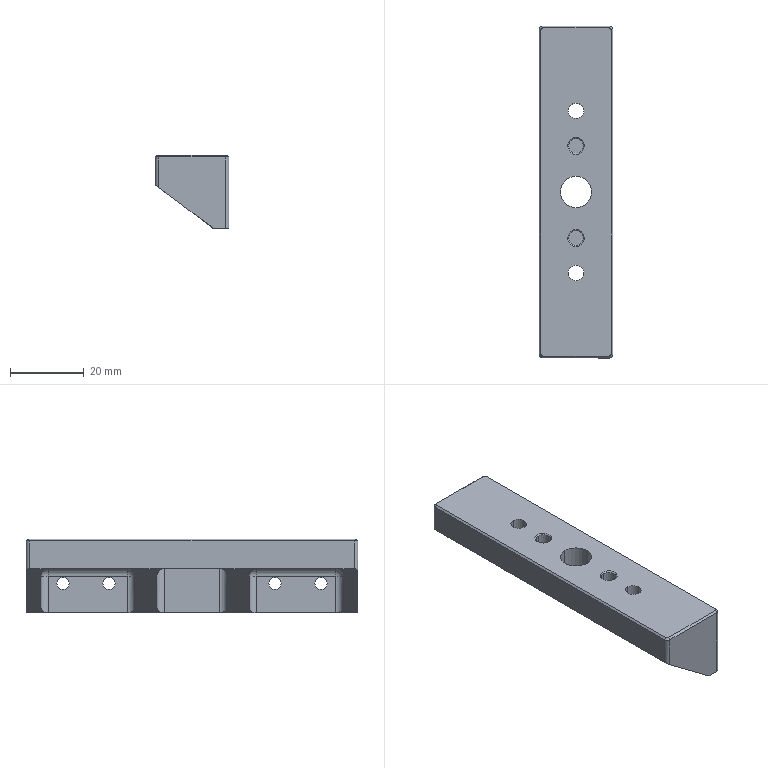NC program | NX | posted with a generic post | part box 20 x 90 x 20 mm
Whole program:
N10 G17 G21 G94 G90
(DRILLING_COPY_1_COPY , TOOL : D6A45)
N12 T01 M6
N14 G54
N16 G17 G0 G90 X-35. Y-2. B0. C0. S5000 M3
N18 G43 Z30. H1
N20 G94 G81 G98 Z-1.75 F350. R3.
N22 X-22.5
N24 X22.5
N26 X35.
N28 G80
N30 G0 X35. Y-2. Z30.
(DRILLING_COPY_1_COPY_COPY , TOOL : D6A45)
N32 X-12.5
N34 G81 Z-2.3 F350. R3.
N36 X12.5
N38 G80
N40 G0 X12.5 Y-2. Z30.
N42 M5
(DRILLING_COPY_COPY_COPY , TOOL : 3.3ZT)
N44 T03 M6
N46 G54
N48 G17 G0 G90 X-35. Y-2. B0. C0. S2000 M3
N50 G43 Z30. H3
N52 G94 G83 G98 Z-6.491 F120. Q2. R3.
N54 X-22.5
N56 X22.5
N58 X35.
N60 G80
N62 G0 X35. Y-2. Z30.
N64 M5
(HOLE_MILLING_COPY_COPY_1 , TOOL : D3)
N66 T17 M6
N68 G54
N70 G17 G0 G90 X-12.5 Y-2. B0. C0. S9500 M3
N72 G43 Z30. H17
N74 Z0.5
N76 G41 G94 G1 X-12.473 Y-2.096 F1200. D17
N78 G3 X-12.05 Y-2. R0.222
N80 X-12.05 Y-2. Z0.25 I-0.45 J0.
N82 X-12.05 Y-2. Z0. I-0.45 J0.
N84 X-12.05 Y-2. Z-0.25 I-0.45 J0.
N86 X-12.05 Y-2. Z-0.5 I-0.45 J0.
N88 X-12.05 Y-2. Z-0.75 I-0.45 J0.
N90 X-12.05 Y-2. Z-1. I-0.45 J0.
N92 X-12.05 Y-2. Z-1.25 I-0.45 J0.
N94 X-12.05 Y-2. Z-1.5 I-0.45 J0.
N96 X-12.05 Y-2. Z-1.75 I-0.45 J0.
N98 X-12.05 Y-2. Z-2. I-0.45 J0.
N100 X-12.05 Y-2. Z-2.25 I-0.45 J0.
N102 X-12.05 Y-2. Z-2.5 I-0.45 J0.
N104 X-12.05 Y-2. Z-2.75 I-0.45 J0.
N106 X-12.05 Y-2. Z-3. I-0.45 J0.
N108 X-12.05 Y-2. Z-3.25 I-0.45 J0.
N110 X-12.05 Y-2. Z-3.5 I-0.45 J0.
N112 X-12.05 Y-2. Z-3.75 I-0.45 J0.
N114 X-12.05 Y-2. Z-4. I-0.45 J0.
N116 X-12.5 Y-1.55 R0.45
N118 X-12.05 Y-2. R-0.45
N120 X-12.473 Y-1.904 R0.222
N122 G40
N124 G1 X-12.5 Y-2.
N126 G0 Z30.
N128 X12.5
N130 Z0.5
N132 G41 G1 X12.527 Y-2.096
N134 G3 X12.95 Y-2. R0.222
N136 X12.95 Y-2. Z0.25 I-0.45 J0.
N138 X12.95 Y-2. Z0. I-0.45 J0.
N140 X12.95 Y-2. Z-0.25 I-0.45 J0.
N142 X12.95 Y-2. Z-0.5 I-0.45 J0.
N144 X12.95 Y-2. Z-0.75 I-0.45 J0.
N146 X12.95 Y-2. Z-1. I-0.45 J0.
N148 X12.95 Y-2. Z-1.25 I-0.45 J0.
N150 X12.95 Y-2. Z-1.5 I-0.45 J0.
N152 X12.95 Y-2. Z-1.75 I-0.45 J0.
N154 X12.95 Y-2. Z-2. I-0.45 J0.
N156 X12.95 Y-2. Z-2.25 I-0.45 J0.
N158 X12.95 Y-2. Z-2.5 I-0.45 J0.
N160 X12.95 Y-2. Z-2.75 I-0.45 J0.
N162 X12.95 Y-2. Z-3. I-0.45 J0.
N164 X12.95 Y-2. Z-3.25 I-0.45 J0.
N166 X12.95 Y-2. Z-3.5 I-0.45 J0.
N168 X12.95 Y-2. Z-3.75 I-0.45 J0.
N170 X12.95 Y-2. Z-4. I-0.45 J0.
N172 X12.5 Y-1.55 R0.45
N174 X12.95 Y-2. R-0.45
N176 X12.527 Y-1.904 R0.222
N178 G40
N180 G1 X12.5 Y-2.
N182 G0 Z30.
N184 M5
N186 M2